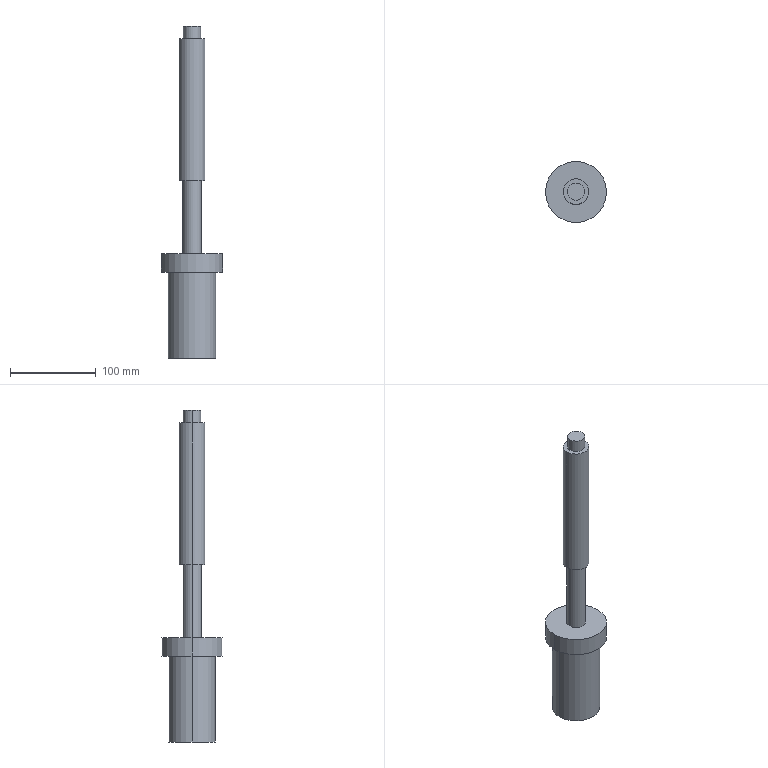Part | SolidWorks | features ICE 4, Extrusion 1 | 1 solid | 19 faces | box 71 x 71 x 386.35 mm | volume 379556 mm3 | cylinder 12 | plane 7 | commonest cylinder face diameters 20 x2 22 x2 30 x2 35 x2 55 x2 71 x2
STEP:
#1=CARTESIAN_POINT('',(10.,0.,386.35));
#2=VERTEX_POINT('',#1);
#3=CARTESIAN_POINT('',(-10.,0.,386.35));
#4=VERTEX_POINT('',#3);
#5=CARTESIAN_POINT('',(0.,0.,386.35));
#6=DIRECTION('',(0.,0.,1.));
#7=DIRECTION('',(1.,0.,0.));
#8=AXIS2_PLACEMENT_3D('',#5,#6,#7);
#9=CIRCLE('',#8,10.);
#10=EDGE_CURVE('',#2,#4,#9,.T.);
#11=ORIENTED_EDGE('',*,*,#10,.F.);
#12=CARTESIAN_POINT('',(10.,0.,371.35));
#13=VERTEX_POINT('',#12);
#14=CARTESIAN_POINT('',(10.,0.,386.35));
#15=DIRECTION('',(0.,0.,-1.));
#16=VECTOR('',#15,1000.);
#17=LINE('',#14,#16);
#18=EDGE_CURVE('',#2,#13,#17,.T.);
#19=ORIENTED_EDGE('',*,*,#18,.T.);
#20=CARTESIAN_POINT('',(-10.,0.,371.35));
#21=VERTEX_POINT('',#20);
#22=CARTESIAN_POINT('',(0.,0.,371.35));
#23=DIRECTION('',(0.,0.,1.));
#24=DIRECTION('',(1.,0.,0.));
#25=AXIS2_PLACEMENT_3D('',#22,#23,#24);
#26=CIRCLE('',#25,10.);
#27=EDGE_CURVE('',#13,#21,#26,.T.);
#28=ORIENTED_EDGE('',*,*,#27,.T.);
#29=CARTESIAN_POINT('',(-10.,0.,386.35));
#30=DIRECTION('',(0.,0.,-1.));
#31=VECTOR('',#30,1000.);
#32=LINE('',#29,#31);
#33=EDGE_CURVE('',#4,#21,#32,.T.);
#34=ORIENTED_EDGE('',*,*,#33,.F.);
#35=EDGE_LOOP('',(#11,#19,#28,#34));
#36=FACE_OUTER_BOUND('',#35,.T.);
#37=CARTESIAN_POINT('',(0.,0.,386.35));
#38=DIRECTION('',(0.,0.,-1.));
#39=DIRECTION('',(-1.,0.,0.));
#40=AXIS2_PLACEMENT_3D('',#37,#38,#39);
#41=CYLINDRICAL_SURFACE('',#40,10.);
#42=ADVANCED_FACE('',(#36),#41,.T.);
#43=CARTESIAN_POINT('',(15.,0.,371.35));
#44=VERTEX_POINT('',#43);
#45=CARTESIAN_POINT('',(-15.,0.,371.35));
#46=VERTEX_POINT('',#45);
#47=CARTESIAN_POINT('',(0.,0.,371.35));
#48=DIRECTION('',(0.,0.,1.));
#49=DIRECTION('',(1.,0.,0.));
#50=AXIS2_PLACEMENT_3D('',#47,#48,#49);
#51=CIRCLE('',#50,15.);
#52=EDGE_CURVE('',#44,#46,#51,.T.);
#53=ORIENTED_EDGE('',*,*,#52,.F.);
#54=CARTESIAN_POINT('',(15.,0.,206.35));
#55=VERTEX_POINT('',#54);
#56=CARTESIAN_POINT('',(15.,0.,371.35));
#57=DIRECTION('',(0.,0.,-1.));
#58=VECTOR('',#57,1000.);
#59=LINE('',#56,#58);
#60=EDGE_CURVE('',#44,#55,#59,.T.);
#61=ORIENTED_EDGE('',*,*,#60,.T.);
#62=CARTESIAN_POINT('',(-15.,0.,206.35));
#63=VERTEX_POINT('',#62);
#64=CARTESIAN_POINT('',(0.,0.,206.35));
#65=DIRECTION('',(0.,0.,1.));
#66=DIRECTION('',(1.,0.,0.));
#67=AXIS2_PLACEMENT_3D('',#64,#65,#66);
#68=CIRCLE('',#67,15.);
#69=EDGE_CURVE('',#55,#63,#68,.T.);
#70=ORIENTED_EDGE('',*,*,#69,.T.);
#71=CARTESIAN_POINT('',(-15.,0.,371.35));
#72=DIRECTION('',(0.,0.,-1.));
#73=VECTOR('',#72,1000.);
#74=LINE('',#71,#73);
#75=EDGE_CURVE('',#46,#63,#74,.T.);
#76=ORIENTED_EDGE('',*,*,#75,.F.);
#77=EDGE_LOOP('',(#53,#61,#70,#76));
#78=FACE_OUTER_BOUND('',#77,.T.);
#79=CARTESIAN_POINT('',(0.,0.,371.35));
#80=DIRECTION('',(0.,0.,-1.));
#81=DIRECTION('',(-1.,0.,0.));
#82=AXIS2_PLACEMENT_3D('',#79,#80,#81);
#83=CYLINDRICAL_SURFACE('',#82,15.);
#84=ADVANCED_FACE('',(#78),#83,.T.);
#85=CARTESIAN_POINT('',(11.,0.,206.35));
#86=VERTEX_POINT('',#85);
#87=CARTESIAN_POINT('',(-11.,0.,206.35));
#88=VERTEX_POINT('',#87);
#89=CARTESIAN_POINT('',(0.,0.,206.35));
#90=DIRECTION('',(0.,0.,1.));
#91=DIRECTION('',(1.,0.,0.));
#92=AXIS2_PLACEMENT_3D('',#89,#90,#91);
#93=CIRCLE('',#92,11.);
#94=EDGE_CURVE('',#86,#88,#93,.T.);
#95=ORIENTED_EDGE('',*,*,#94,.F.);
#96=CARTESIAN_POINT('',(11.,0.,121.35));
#97=VERTEX_POINT('',#96);
#98=CARTESIAN_POINT('',(11.,0.,206.35));
#99=DIRECTION('',(0.,0.,-1.));
#100=VECTOR('',#99,1000.);
#101=LINE('',#98,#100);
#102=EDGE_CURVE('',#86,#97,#101,.T.);
#103=ORIENTED_EDGE('',*,*,#102,.T.);
#104=CARTESIAN_POINT('',(-11.,0.,121.35));
#105=VERTEX_POINT('',#104);
#106=CARTESIAN_POINT('',(0.,0.,121.35));
#107=DIRECTION('',(0.,0.,1.));
#108=DIRECTION('',(1.,0.,0.));
#109=AXIS2_PLACEMENT_3D('',#106,#107,#108);
#110=CIRCLE('',#109,11.);
#111=EDGE_CURVE('',#97,#105,#110,.T.);
#112=ORIENTED_EDGE('',*,*,#111,.T.);
#113=CARTESIAN_POINT('',(-11.,0.,206.35));
#114=DIRECTION('',(0.,0.,-1.));
#115=VECTOR('',#114,1000.);
#116=LINE('',#113,#115);
#117=EDGE_CURVE('',#88,#105,#116,.T.);
#118=ORIENTED_EDGE('',*,*,#117,.F.);
#119=EDGE_LOOP('',(#95,#103,#112,#118));
#120=FACE_OUTER_BOUND('',#119,.T.);
#121=CARTESIAN_POINT('',(0.,0.,206.35));
#122=DIRECTION('',(0.,0.,-1.));
#123=DIRECTION('',(-1.,0.,0.));
#124=AXIS2_PLACEMENT_3D('',#121,#122,#123);
#125=CYLINDRICAL_SURFACE('',#124,11.);
#126=ADVANCED_FACE('',(#120),#125,.T.);
#127=CARTESIAN_POINT('',(35.5,0.,121.35));
#128=VERTEX_POINT('',#127);
#129=CARTESIAN_POINT('',(-35.5,0.,121.35));
#130=VERTEX_POINT('',#129);
#131=CARTESIAN_POINT('',(0.,0.,121.35));
#132=DIRECTION('',(0.,0.,1.));
#133=DIRECTION('',(1.,0.,0.));
#134=AXIS2_PLACEMENT_3D('',#131,#132,#133);
#135=CIRCLE('',#134,35.5);
#136=EDGE_CURVE('',#128,#130,#135,.T.);
#137=ORIENTED_EDGE('',*,*,#136,.F.);
#138=CARTESIAN_POINT('',(35.5,0.,100.));
#139=VERTEX_POINT('',#138);
#140=CARTESIAN_POINT('',(35.5,0.,121.35));
#141=DIRECTION('',(0.,0.,-1.));
#142=VECTOR('',#141,1000.);
#143=LINE('',#140,#142);
#144=EDGE_CURVE('',#128,#139,#143,.T.);
#145=ORIENTED_EDGE('',*,*,#144,.T.);
#146=CARTESIAN_POINT('',(-35.5,0.,100.));
#147=VERTEX_POINT('',#146);
#148=CARTESIAN_POINT('',(0.,0.,100.));
#149=DIRECTION('',(0.,0.,1.));
#150=DIRECTION('',(1.,0.,0.));
#151=AXIS2_PLACEMENT_3D('',#148,#149,#150);
#152=CIRCLE('',#151,35.5);
#153=EDGE_CURVE('',#139,#147,#152,.T.);
#154=ORIENTED_EDGE('',*,*,#153,.T.);
#155=CARTESIAN_POINT('',(-35.5,0.,121.35));
#156=DIRECTION('',(0.,0.,-1.));
#157=VECTOR('',#156,1000.);
#158=LINE('',#155,#157);
#159=EDGE_CURVE('',#130,#147,#158,.T.);
#160=ORIENTED_EDGE('',*,*,#159,.F.);
#161=EDGE_LOOP('',(#137,#145,#154,#160));
#162=FACE_OUTER_BOUND('',#161,.T.);
#163=CARTESIAN_POINT('',(0.,0.,121.35));
#164=DIRECTION('',(0.,0.,-1.));
#165=DIRECTION('',(-1.,0.,0.));
#166=AXIS2_PLACEMENT_3D('',#163,#164,#165);
#167=CYLINDRICAL_SURFACE('',#166,35.5);
#168=ADVANCED_FACE('',(#162),#167,.T.);
#169=CARTESIAN_POINT('',(-17.5,0.,100.));
#170=VERTEX_POINT('',#169);
#171=CARTESIAN_POINT('',(17.5,0.,100.));
#172=VERTEX_POINT('',#171);
#173=CARTESIAN_POINT('',(0.,0.,100.));
#174=DIRECTION('',(0.,0.,1.));
#175=DIRECTION('',(1.,0.,0.));
#176=AXIS2_PLACEMENT_3D('',#173,#174,#175);
#177=CIRCLE('',#176,17.5);
#178=EDGE_CURVE('',#170,#172,#177,.T.);
#179=ORIENTED_EDGE('',*,*,#178,.T.);
#180=CARTESIAN_POINT('',(17.5,0.,0.));
#181=VERTEX_POINT('',#180);
#182=CARTESIAN_POINT('',(17.5,0.,100.));
#183=DIRECTION('',(0.,0.,-1.));
#184=VECTOR('',#183,1000.);
#185=LINE('',#182,#184);
#186=EDGE_CURVE('',#172,#181,#185,.T.);
#187=ORIENTED_EDGE('',*,*,#186,.T.);
#188=CARTESIAN_POINT('',(-17.5,0.,0.));
#189=VERTEX_POINT('',#188);
#190=CARTESIAN_POINT('',(0.,0.,0.));
#191=DIRECTION('',(0.,0.,1.));
#192=DIRECTION('',(1.,0.,0.));
#193=AXIS2_PLACEMENT_3D('',#190,#191,#192);
#194=CIRCLE('',#193,17.5);
#195=EDGE_CURVE('',#189,#181,#194,.T.);
#196=ORIENTED_EDGE('',*,*,#195,.F.);
#197=CARTESIAN_POINT('',(-17.5,0.,100.));
#198=DIRECTION('',(0.,0.,-1.));
#199=VECTOR('',#198,1000.);
#200=LINE('',#197,#199);
#201=EDGE_CURVE('',#170,#189,#200,.T.);
#202=ORIENTED_EDGE('',*,*,#201,.F.);
#203=EDGE_LOOP('',(#179,#187,#196,#202));
#204=FACE_OUTER_BOUND('',#203,.T.);
#205=CARTESIAN_POINT('',(0.,0.,100.));
#206=DIRECTION('',(0.,0.,-1.));
#207=DIRECTION('',(-1.,0.,0.));
#208=AXIS2_PLACEMENT_3D('',#205,#206,#207);
#209=CYLINDRICAL_SURFACE('',#208,17.5);
#210=ADVANCED_FACE('',(#204),#209,.F.);
#211=CARTESIAN_POINT('',(27.5,0.,100.));
#212=VERTEX_POINT('',#211);
#213=CARTESIAN_POINT('',(-27.5,0.,100.));
#214=VERTEX_POINT('',#213);
#215=CARTESIAN_POINT('',(0.,0.,100.));
#216=DIRECTION('',(0.,0.,1.));
#217=DIRECTION('',(1.,0.,0.));
#218=AXIS2_PLACEMENT_3D('',#215,#216,#217);
#219=CIRCLE('',#218,27.5);
#220=EDGE_CURVE('',#212,#214,#219,.T.);
#221=ORIENTED_EDGE('',*,*,#220,.F.);
#222=CARTESIAN_POINT('',(27.5,0.,0.));
#223=VERTEX_POINT('',#222);
#224=CARTESIAN_POINT('',(27.5,0.,100.));
#225=DIRECTION('',(0.,0.,-1.));
#226=VECTOR('',#225,1000.);
#227=LINE('',#224,#226);
#228=EDGE_CURVE('',#212,#223,#227,.T.);
#229=ORIENTED_EDGE('',*,*,#228,.T.);
#230=CARTESIAN_POINT('',(-27.5,0.,0.));
#231=VERTEX_POINT('',#230);
#232=CARTESIAN_POINT('',(0.,0.,0.));
#233=DIRECTION('',(0.,0.,1.));
#234=DIRECTION('',(1.,0.,0.));
#235=AXIS2_PLACEMENT_3D('',#232,#233,#234);
#236=CIRCLE('',#235,27.5);
#237=EDGE_CURVE('',#223,#231,#236,.T.);
#238=ORIENTED_EDGE('',*,*,#237,.T.);
#239=CARTESIAN_POINT('',(-27.5,0.,100.));
#240=DIRECTION('',(0.,0.,-1.));
#241=VECTOR('',#240,1000.);
#242=LINE('',#239,#241);
#243=EDGE_CURVE('',#214,#231,#242,.T.);
#244=ORIENTED_EDGE('',*,*,#243,.F.);
#245=EDGE_LOOP('',(#221,#229,#238,#244));
#246=FACE_OUTER_BOUND('',#245,.T.);
#247=CARTESIAN_POINT('',(0.,0.,100.));
#248=DIRECTION('',(0.,0.,-1.));
#249=DIRECTION('',(-1.,0.,0.));
#250=AXIS2_PLACEMENT_3D('',#247,#248,#249);
#251=CYLINDRICAL_SURFACE('',#250,27.5);
#252=ADVANCED_FACE('',(#246),#251,.T.);
#253=CARTESIAN_POINT('',(0.,0.,0.));
#254=DIRECTION('',(0.,0.,1.));
#255=DIRECTION('',(1.,0.,0.));
#256=AXIS2_PLACEMENT_3D('',#253,#254,#255);
#257=CIRCLE('',#256,27.5);
#258=EDGE_CURVE('',#231,#223,#257,.T.);
#259=ORIENTED_EDGE('',*,*,#258,.F.);
#260=ORIENTED_EDGE('',*,*,#237,.F.);
#261=EDGE_LOOP('',(#259,#260));
#262=FACE_OUTER_BOUND('',#261,.T.);
#263=ORIENTED_EDGE('',*,*,#195,.T.);
#264=CARTESIAN_POINT('',(0.,0.,0.));
#265=DIRECTION('',(0.,0.,1.));
#266=DIRECTION('',(1.,0.,0.));
#267=AXIS2_PLACEMENT_3D('',#264,#265,#266);
#268=CIRCLE('',#267,17.5);
#269=EDGE_CURVE('',#181,#189,#268,.T.);
#270=ORIENTED_EDGE('',*,*,#269,.T.);
#271=EDGE_LOOP('',(#263,#270));
#272=FACE_BOUND('',#271,.T.);
#273=CARTESIAN_POINT('',(0.,0.,0.));
#274=DIRECTION('',(0.,0.,1.));
#275=DIRECTION('',(1.,0.,0.));
#276=AXIS2_PLACEMENT_3D('',#273,#274,#275);
#277=PLANE('',#276);
#278=ADVANCED_FACE('',(#262,#272),#277,.F.);
#279=ORIENTED_EDGE('',*,*,#228,.F.);
#280=CARTESIAN_POINT('',(0.,0.,100.));
#281=DIRECTION('',(0.,0.,1.));
#282=DIRECTION('',(1.,0.,0.));
#283=AXIS2_PLACEMENT_3D('',#280,#281,#282);
#284=CIRCLE('',#283,27.5);
#285=EDGE_CURVE('',#214,#212,#284,.T.);
#286=ORIENTED_EDGE('',*,*,#285,.F.);
#287=ORIENTED_EDGE('',*,*,#243,.T.);
#288=ORIENTED_EDGE('',*,*,#258,.T.);
#289=EDGE_LOOP('',(#279,#286,#287,#288));
#290=FACE_OUTER_BOUND('',#289,.T.);
#291=CARTESIAN_POINT('',(0.,0.,100.));
#292=DIRECTION('',(0.,0.,-1.));
#293=DIRECTION('',(-1.,0.,0.));
#294=AXIS2_PLACEMENT_3D('',#291,#292,#293);
#295=CYLINDRICAL_SURFACE('',#294,27.5);
#296=ADVANCED_FACE('',(#290),#295,.T.);
#297=ORIENTED_EDGE('',*,*,#186,.F.);
#298=CARTESIAN_POINT('',(0.,0.,100.));
#299=DIRECTION('',(0.,0.,1.));
#300=DIRECTION('',(1.,0.,0.));
#301=AXIS2_PLACEMENT_3D('',#298,#299,#300);
#302=CIRCLE('',#301,17.5);
#303=EDGE_CURVE('',#172,#170,#302,.T.);
#304=ORIENTED_EDGE('',*,*,#303,.T.);
#305=ORIENTED_EDGE('',*,*,#201,.T.);
#306=ORIENTED_EDGE('',*,*,#269,.F.);
#307=EDGE_LOOP('',(#297,#304,#305,#306));
#308=FACE_OUTER_BOUND('',#307,.T.);
#309=CARTESIAN_POINT('',(0.,0.,100.));
#310=DIRECTION('',(0.,0.,-1.));
#311=DIRECTION('',(-1.,0.,0.));
#312=AXIS2_PLACEMENT_3D('',#309,#310,#311);
#313=CYLINDRICAL_SURFACE('',#312,17.5);
#314=ADVANCED_FACE('',(#308),#313,.F.);
#315=ORIENTED_EDGE('',*,*,#178,.F.);
#316=ORIENTED_EDGE('',*,*,#303,.F.);
#317=EDGE_LOOP('',(#315,#316));
#318=FACE_OUTER_BOUND('',#317,.T.);
#319=CARTESIAN_POINT('',(0.,0.,100.));
#320=DIRECTION('',(0.,0.,1.));
#321=DIRECTION('',(1.,0.,0.));
#322=AXIS2_PLACEMENT_3D('',#319,#320,#321);
#323=PLANE('',#322);
#324=ADVANCED_FACE('',(#318),#323,.F.);
#325=ORIENTED_EDGE('',*,*,#144,.F.);
#326=CARTESIAN_POINT('',(0.,0.,121.35));
#327=DIRECTION('',(0.,0.,1.));
#328=DIRECTION('',(1.,0.,0.));
#329=AXIS2_PLACEMENT_3D('',#326,#327,#328);
#330=CIRCLE('',#329,35.5);
#331=EDGE_CURVE('',#130,#128,#330,.T.);
#332=ORIENTED_EDGE('',*,*,#331,.F.);
#333=ORIENTED_EDGE('',*,*,#159,.T.);
#334=CARTESIAN_POINT('',(0.,0.,100.));
#335=DIRECTION('',(0.,0.,1.));
#336=DIRECTION('',(1.,0.,0.));
#337=AXIS2_PLACEMENT_3D('',#334,#335,#336);
#338=CIRCLE('',#337,35.5);
#339=EDGE_CURVE('',#147,#139,#338,.T.);
#340=ORIENTED_EDGE('',*,*,#339,.T.);
#341=EDGE_LOOP('',(#325,#332,#333,#340));
#342=FACE_OUTER_BOUND('',#341,.T.);
#343=CARTESIAN_POINT('',(0.,0.,121.35));
#344=DIRECTION('',(0.,0.,-1.));
#345=DIRECTION('',(-1.,0.,0.));
#346=AXIS2_PLACEMENT_3D('',#343,#344,#345);
#347=CYLINDRICAL_SURFACE('',#346,35.5);
#348=ADVANCED_FACE('',(#342),#347,.T.);
#349=CARTESIAN_POINT('',(0.,0.,121.35));
#350=DIRECTION('',(0.,0.,1.));
#351=DIRECTION('',(1.,0.,0.));
#352=AXIS2_PLACEMENT_3D('',#349,#350,#351);
#353=CIRCLE('',#352,11.);
#354=EDGE_CURVE('',#105,#97,#353,.T.);
#355=ORIENTED_EDGE('',*,*,#354,.F.);
#356=ORIENTED_EDGE('',*,*,#111,.F.);
#357=EDGE_LOOP('',(#355,#356));
#358=FACE_BOUND('',#357,.T.);
#359=ORIENTED_EDGE('',*,*,#331,.T.);
#360=ORIENTED_EDGE('',*,*,#136,.T.);
#361=EDGE_LOOP('',(#359,#360));
#362=FACE_OUTER_BOUND('',#361,.T.);
#363=CARTESIAN_POINT('',(0.,0.,121.35));
#364=DIRECTION('',(0.,0.,1.));
#365=DIRECTION('',(1.,0.,0.));
#366=AXIS2_PLACEMENT_3D('',#363,#364,#365);
#367=PLANE('',#366);
#368=ADVANCED_FACE('',(#358,#362),#367,.T.);
#369=ORIENTED_EDGE('',*,*,#285,.T.);
#370=ORIENTED_EDGE('',*,*,#220,.T.);
#371=EDGE_LOOP('',(#369,#370));
#372=FACE_BOUND('',#371,.T.);
#373=ORIENTED_EDGE('',*,*,#339,.F.);
#374=ORIENTED_EDGE('',*,*,#153,.F.);
#375=EDGE_LOOP('',(#373,#374));
#376=FACE_OUTER_BOUND('',#375,.T.);
#377=CARTESIAN_POINT('',(0.,0.,100.));
#378=DIRECTION('',(0.,0.,1.));
#379=DIRECTION('',(1.,0.,0.));
#380=AXIS2_PLACEMENT_3D('',#377,#378,#379);
#381=PLANE('',#380);
#382=ADVANCED_FACE('',(#372,#376),#381,.F.);
#383=ORIENTED_EDGE('',*,*,#102,.F.);
#384=CARTESIAN_POINT('',(0.,0.,206.35));
#385=DIRECTION('',(0.,0.,1.));
#386=DIRECTION('',(1.,0.,0.));
#387=AXIS2_PLACEMENT_3D('',#384,#385,#386);
#388=CIRCLE('',#387,11.);
#389=EDGE_CURVE('',#88,#86,#388,.T.);
#390=ORIENTED_EDGE('',*,*,#389,.F.);
#391=ORIENTED_EDGE('',*,*,#117,.T.);
#392=ORIENTED_EDGE('',*,*,#354,.T.);
#393=EDGE_LOOP('',(#383,#390,#391,#392));
#394=FACE_OUTER_BOUND('',#393,.T.);
#395=CARTESIAN_POINT('',(0.,0.,206.35));
#396=DIRECTION('',(0.,0.,-1.));
#397=DIRECTION('',(-1.,0.,0.));
#398=AXIS2_PLACEMENT_3D('',#395,#396,#397);
#399=CYLINDRICAL_SURFACE('',#398,11.);
#400=ADVANCED_FACE('',(#394),#399,.T.);
#401=ORIENTED_EDGE('',*,*,#60,.F.);
#402=CARTESIAN_POINT('',(0.,0.,371.35));
#403=DIRECTION('',(0.,0.,1.));
#404=DIRECTION('',(1.,0.,0.));
#405=AXIS2_PLACEMENT_3D('',#402,#403,#404);
#406=CIRCLE('',#405,15.);
#407=EDGE_CURVE('',#46,#44,#406,.T.);
#408=ORIENTED_EDGE('',*,*,#407,.F.);
#409=ORIENTED_EDGE('',*,*,#75,.T.);
#410=CARTESIAN_POINT('',(0.,0.,206.35));
#411=DIRECTION('',(0.,0.,1.));
#412=DIRECTION('',(1.,0.,0.));
#413=AXIS2_PLACEMENT_3D('',#410,#411,#412);
#414=CIRCLE('',#413,15.);
#415=EDGE_CURVE('',#63,#55,#414,.T.);
#416=ORIENTED_EDGE('',*,*,#415,.T.);
#417=EDGE_LOOP('',(#401,#408,#409,#416));
#418=FACE_OUTER_BOUND('',#417,.T.);
#419=CARTESIAN_POINT('',(0.,0.,371.35));
#420=DIRECTION('',(0.,0.,-1.));
#421=DIRECTION('',(-1.,0.,0.));
#422=AXIS2_PLACEMENT_3D('',#419,#420,#421);
#423=CYLINDRICAL_SURFACE('',#422,15.);
#424=ADVANCED_FACE('',(#418),#423,.T.);
#425=CARTESIAN_POINT('',(0.,0.,371.35));
#426=DIRECTION('',(0.,0.,1.));
#427=DIRECTION('',(1.,0.,0.));
#428=AXIS2_PLACEMENT_3D('',#425,#426,#427);
#429=CIRCLE('',#428,10.);
#430=EDGE_CURVE('',#21,#13,#429,.T.);
#431=ORIENTED_EDGE('',*,*,#430,.F.);
#432=ORIENTED_EDGE('',*,*,#27,.F.);
#433=EDGE_LOOP('',(#431,#432));
#434=FACE_BOUND('',#433,.T.);
#435=ORIENTED_EDGE('',*,*,#407,.T.);
#436=ORIENTED_EDGE('',*,*,#52,.T.);
#437=EDGE_LOOP('',(#435,#436));
#438=FACE_OUTER_BOUND('',#437,.T.);
#439=CARTESIAN_POINT('',(0.,0.,371.35));
#440=DIRECTION('',(0.,0.,1.));
#441=DIRECTION('',(1.,0.,0.));
#442=AXIS2_PLACEMENT_3D('',#439,#440,#441);
#443=PLANE('',#442);
#444=ADVANCED_FACE('',(#434,#438),#443,.T.);
#445=ORIENTED_EDGE('',*,*,#389,.T.);
#446=ORIENTED_EDGE('',*,*,#94,.T.);
#447=EDGE_LOOP('',(#445,#446));
#448=FACE_BOUND('',#447,.T.);
#449=ORIENTED_EDGE('',*,*,#415,.F.);
#450=ORIENTED_EDGE('',*,*,#69,.F.);
#451=EDGE_LOOP('',(#449,#450));
#452=FACE_OUTER_BOUND('',#451,.T.);
#453=CARTESIAN_POINT('',(0.,0.,206.35));
#454=DIRECTION('',(0.,0.,1.));
#455=DIRECTION('',(1.,0.,0.));
#456=AXIS2_PLACEMENT_3D('',#453,#454,#455);
#457=PLANE('',#456);
#458=ADVANCED_FACE('',(#448,#452),#457,.F.);
#459=ORIENTED_EDGE('',*,*,#18,.F.);
#460=CARTESIAN_POINT('',(0.,0.,386.35));
#461=DIRECTION('',(0.,0.,1.));
#462=DIRECTION('',(1.,0.,0.));
#463=AXIS2_PLACEMENT_3D('',#460,#461,#462);
#464=CIRCLE('',#463,10.);
#465=EDGE_CURVE('',#4,#2,#464,.T.);
#466=ORIENTED_EDGE('',*,*,#465,.F.);
#467=ORIENTED_EDGE('',*,*,#33,.T.);
#468=ORIENTED_EDGE('',*,*,#430,.T.);
#469=EDGE_LOOP('',(#459,#466,#467,#468));
#470=FACE_OUTER_BOUND('',#469,.T.);
#471=CARTESIAN_POINT('',(0.,0.,386.35));
#472=DIRECTION('',(0.,0.,-1.));
#473=DIRECTION('',(-1.,0.,0.));
#474=AXIS2_PLACEMENT_3D('',#471,#472,#473);
#475=CYLINDRICAL_SURFACE('',#474,10.);
#476=ADVANCED_FACE('',(#470),#475,.T.);
#477=ORIENTED_EDGE('',*,*,#465,.T.);
#478=ORIENTED_EDGE('',*,*,#10,.T.);
#479=EDGE_LOOP('',(#477,#478));
#480=FACE_OUTER_BOUND('',#479,.T.);
#481=CARTESIAN_POINT('',(0.,0.,386.35));
#482=DIRECTION('',(0.,0.,1.));
#483=DIRECTION('',(1.,0.,0.));
#484=AXIS2_PLACEMENT_3D('',#481,#482,#483);
#485=PLANE('',#484);
#486=ADVANCED_FACE('',(#480),#485,.T.);
#487=CLOSED_SHELL('',(#42,#84,#126,#168,#210,#252,#278,#296,#314,#324,#348,#368,#382,#400,#424,#444,#458,#476,#486));
#488=MANIFOLD_SOLID_BREP('',#487);
#489=CARTESIAN_POINT('',(0.,0.,0.));
#490=DIRECTION('',(0.,0.,1.));
#491=DIRECTION('',(1.,0.,0.));
#492=AXIS2_PLACEMENT_3D('',#489,#490,#491);
#493=(LENGTH_UNIT()NAMED_UNIT(*)SI_UNIT(.MILLI.,.METRE.));
#494=UNCERTAINTY_MEASURE_WITH_UNIT(LENGTH_MEASURE(0.00001),#493,'','');
#495=(NAMED_UNIT(*)PLANE_ANGLE_UNIT()SI_UNIT($,.RADIAN.));
#496=(NAMED_UNIT(*)SI_UNIT($,.STERADIAN.)SOLID_ANGLE_UNIT());
#497=(GEOMETRIC_REPRESENTATION_CONTEXT(3)GLOBAL_UNCERTAINTY_ASSIGNED_CONTEXT((#494))GLOBAL_UNIT_ASSIGNED_CONTEXT((#493,#495,#496))REPRESENTATION_CONTEXT('',''));
#498=ADVANCED_BREP_SHAPE_REPRESENTATION('',(#488,#492),#497);